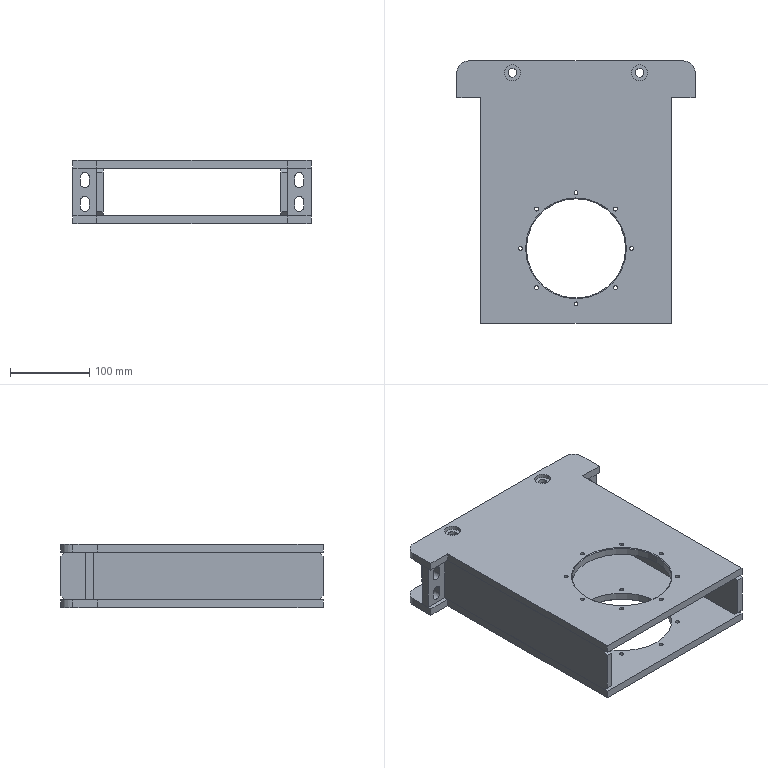Part | SolidWorks | features ICE 11, Chamfer 4, CirPattern 2, HoleWzd 2, LPattern 2, Extrusion 1, Fillet 1, MirrorSolid 1, WeldmentFeature 1 | 6 solids | 136 faces | box 300 x 330 x 80 mm | volume 1723505 mm3 | plane 66 | cylinder 66 | cone 4 | commonest cylinder face diameters 5 x32 11 x16 20 x10 30 x4 125 x4